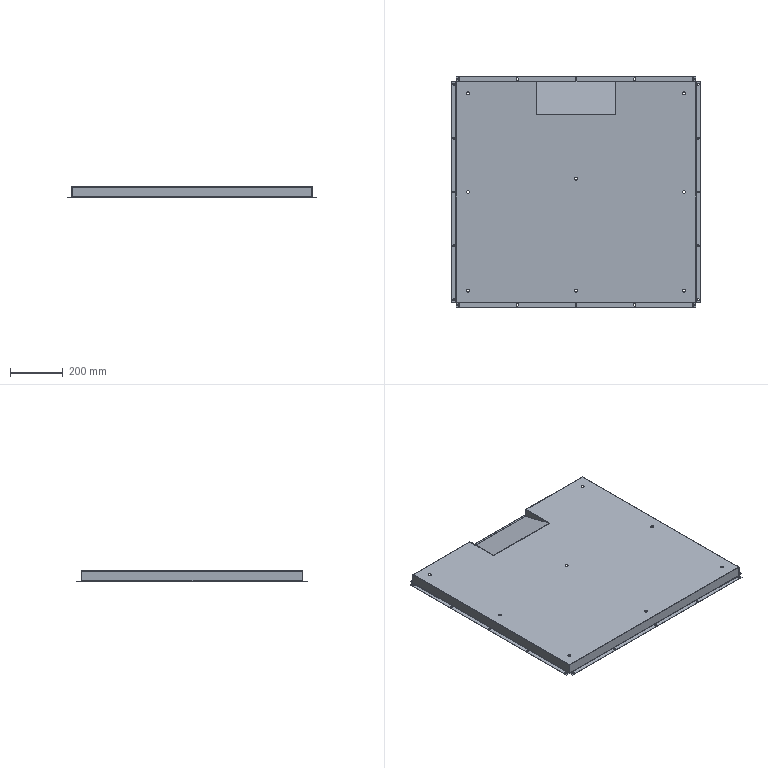Part | 2 solids | 206 faces | box 939 x 869 x 40 mm | volume 941846 mm3 | plane 106 | cylinder 88 | spline 12 | commonest cylinder face diameters 7 x50 11 x16 0.4 x11 2.4 x11